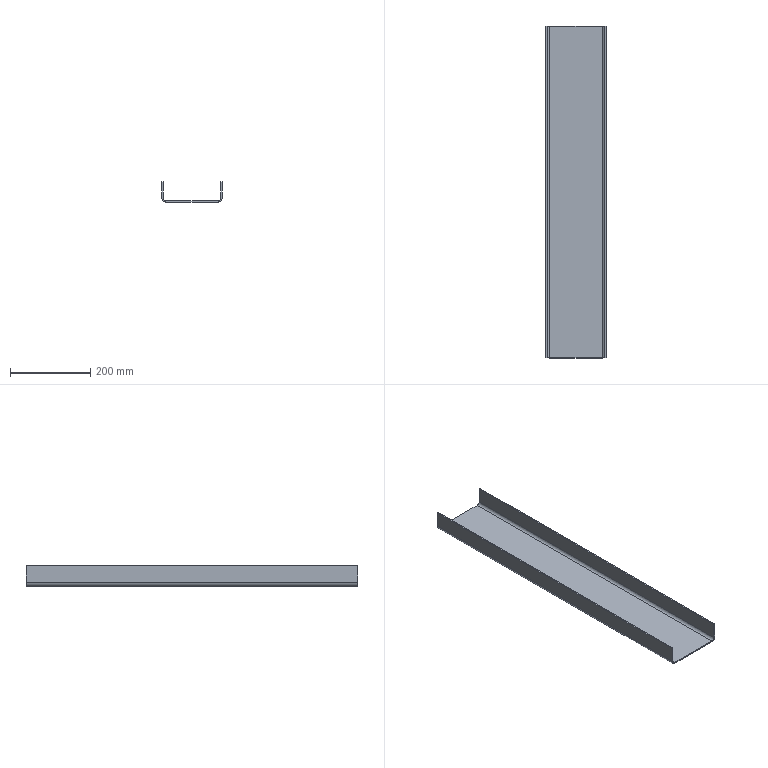Part | SolidWorks | features ExtruThin 1 | 1 solid | 14 faces | box 150 x 827 x 50 mm | volume 587261 mm3 | plane 10 | cylinder 4 | commonest cylinder face diameters 14 x2 20 x2
STEP:
#1=CARTESIAN_POINT('',(-75.,-413.5,-15.));
#2=VERTEX_POINT('',#1);
#3=CARTESIAN_POINT('',(-75.,-413.5,25.));
#4=VERTEX_POINT('',#3);
#5=CARTESIAN_POINT('',(-75.,-413.5,-15.));
#6=DIRECTION('',(0.,0.,1.));
#7=VECTOR('',#6,1000.);
#8=LINE('',#5,#7);
#9=EDGE_CURVE('',#2,#4,#8,.T.);
#10=ORIENTED_EDGE('',*,*,#9,.T.);
#11=CARTESIAN_POINT('',(-75.,413.5,25.));
#12=VERTEX_POINT('',#11);
#13=CARTESIAN_POINT('',(-75.,413.5,25.));
#14=DIRECTION('',(0.,-1.,0.));
#15=VECTOR('',#14,1000.);
#16=LINE('',#13,#15);
#17=EDGE_CURVE('',#12,#4,#16,.T.);
#18=ORIENTED_EDGE('',*,*,#17,.F.);
#19=CARTESIAN_POINT('',(-75.,413.5,-15.));
#20=VERTEX_POINT('',#19);
#21=CARTESIAN_POINT('',(-75.,413.5,-15.));
#22=DIRECTION('',(0.,0.,1.));
#23=VECTOR('',#22,1000.);
#24=LINE('',#21,#23);
#25=EDGE_CURVE('',#20,#12,#24,.T.);
#26=ORIENTED_EDGE('',*,*,#25,.F.);
#27=CARTESIAN_POINT('',(-75.,413.5,-15.));
#28=DIRECTION('',(0.,-1.,0.));
#29=VECTOR('',#28,1000.);
#30=LINE('',#27,#29);
#31=EDGE_CURVE('',#20,#2,#30,.T.);
#32=ORIENTED_EDGE('',*,*,#31,.T.);
#33=EDGE_LOOP('',(#10,#18,#26,#32));
#34=FACE_OUTER_BOUND('',#33,.T.);
#35=CARTESIAN_POINT('',(-75.,413.5,-15.));
#36=DIRECTION('',(1.,0.,0.));
#37=DIRECTION('',(0.,0.,-1.));
#38=AXIS2_PLACEMENT_3D('',#35,#36,#37);
#39=PLANE('',#38);
#40=ADVANCED_FACE('',(#34),#39,.F.);
#41=CARTESIAN_POINT('',(-72.,-413.5,25.));
#42=VERTEX_POINT('',#41);
#43=CARTESIAN_POINT('',(-72.,-413.5,25.));
#44=DIRECTION('',(-1.,0.,0.));
#45=VECTOR('',#44,1000.);
#46=LINE('',#43,#45);
#47=EDGE_CURVE('',#42,#4,#46,.T.);
#48=ORIENTED_EDGE('',*,*,#47,.F.);
#49=CARTESIAN_POINT('',(-72.,413.5,25.));
#50=VERTEX_POINT('',#49);
#51=CARTESIAN_POINT('',(-72.,413.5,25.));
#52=DIRECTION('',(0.,-1.,0.));
#53=VECTOR('',#52,1000.);
#54=LINE('',#51,#53);
#55=EDGE_CURVE('',#50,#42,#54,.T.);
#56=ORIENTED_EDGE('',*,*,#55,.F.);
#57=CARTESIAN_POINT('',(-72.,413.5,25.));
#58=DIRECTION('',(-1.,0.,0.));
#59=VECTOR('',#58,1000.);
#60=LINE('',#57,#59);
#61=EDGE_CURVE('',#50,#12,#60,.T.);
#62=ORIENTED_EDGE('',*,*,#61,.T.);
#63=ORIENTED_EDGE('',*,*,#17,.T.);
#64=EDGE_LOOP('',(#48,#56,#62,#63));
#65=FACE_OUTER_BOUND('',#64,.T.);
#66=CARTESIAN_POINT('',(-72.,413.5,25.));
#67=DIRECTION('',(0.,0.,1.));
#68=DIRECTION('',(1.,0.,0.));
#69=AXIS2_PLACEMENT_3D('',#66,#67,#68);
#70=PLANE('',#69);
#71=ADVANCED_FACE('',(#65),#70,.T.);
#72=CARTESIAN_POINT('',(-72.,-413.5,-15.));
#73=VERTEX_POINT('',#72);
#74=CARTESIAN_POINT('',(-72.,-413.5,-15.));
#75=DIRECTION('',(0.,0.,1.));
#76=VECTOR('',#75,1000.);
#77=LINE('',#74,#76);
#78=EDGE_CURVE('',#73,#42,#77,.T.);
#79=ORIENTED_EDGE('',*,*,#78,.F.);
#80=CARTESIAN_POINT('',(-72.,413.5,-15.));
#81=VERTEX_POINT('',#80);
#82=CARTESIAN_POINT('',(-72.,413.5,-15.));
#83=DIRECTION('',(0.,-1.,0.));
#84=VECTOR('',#83,1000.);
#85=LINE('',#82,#84);
#86=EDGE_CURVE('',#81,#73,#85,.T.);
#87=ORIENTED_EDGE('',*,*,#86,.F.);
#88=CARTESIAN_POINT('',(-72.,413.5,-15.));
#89=DIRECTION('',(0.,0.,1.));
#90=VECTOR('',#89,1000.);
#91=LINE('',#88,#90);
#92=EDGE_CURVE('',#81,#50,#91,.T.);
#93=ORIENTED_EDGE('',*,*,#92,.T.);
#94=ORIENTED_EDGE('',*,*,#55,.T.);
#95=EDGE_LOOP('',(#79,#87,#93,#94));
#96=FACE_OUTER_BOUND('',#95,.T.);
#97=CARTESIAN_POINT('',(-72.,413.5,-15.));
#98=DIRECTION('',(1.,0.,0.));
#99=DIRECTION('',(0.,0.,-1.));
#100=AXIS2_PLACEMENT_3D('',#97,#98,#99);
#101=PLANE('',#100);
#102=ADVANCED_FACE('',(#96),#101,.T.);
#103=CARTESIAN_POINT('',(-65.,-413.5,-22.));
#104=VERTEX_POINT('',#103);
#105=CARTESIAN_POINT('',(-65.,-413.5,-15.));
#106=DIRECTION('',(0.,1.,0.));
#107=DIRECTION('',(1.,0.,0.));
#108=AXIS2_PLACEMENT_3D('',#105,#106,#107);
#109=CIRCLE('',#108,7.);
#110=EDGE_CURVE('',#104,#73,#109,.T.);
#111=ORIENTED_EDGE('',*,*,#110,.F.);
#112=CARTESIAN_POINT('',(-65.,413.5,-22.));
#113=VERTEX_POINT('',#112);
#114=CARTESIAN_POINT('',(-65.,413.5,-22.));
#115=DIRECTION('',(0.,-1.,0.));
#116=VECTOR('',#115,1000.);
#117=LINE('',#114,#116);
#118=EDGE_CURVE('',#113,#104,#117,.T.);
#119=ORIENTED_EDGE('',*,*,#118,.F.);
#120=CARTESIAN_POINT('',(-65.,413.5,-15.));
#121=DIRECTION('',(0.,1.,0.));
#122=DIRECTION('',(1.,0.,0.));
#123=AXIS2_PLACEMENT_3D('',#120,#121,#122);
#124=CIRCLE('',#123,7.);
#125=EDGE_CURVE('',#113,#81,#124,.T.);
#126=ORIENTED_EDGE('',*,*,#125,.T.);
#127=ORIENTED_EDGE('',*,*,#86,.T.);
#128=EDGE_LOOP('',(#111,#119,#126,#127));
#129=FACE_OUTER_BOUND('',#128,.T.);
#130=CARTESIAN_POINT('',(-65.,413.5,-15.));
#131=DIRECTION('',(0.,-1.,0.));
#132=DIRECTION('',(0.,0.,-1.));
#133=AXIS2_PLACEMENT_3D('',#130,#131,#132);
#134=CYLINDRICAL_SURFACE('',#133,7.);
#135=ADVANCED_FACE('',(#129),#134,.F.);
#136=CARTESIAN_POINT('',(65.,-413.5,-22.));
#137=VERTEX_POINT('',#136);
#138=CARTESIAN_POINT('',(-65.,-413.5,-22.));
#139=DIRECTION('',(-1.,0.,0.));
#140=VECTOR('',#139,1000.);
#141=LINE('',#138,#140);
#142=EDGE_CURVE('',#137,#104,#141,.T.);
#143=ORIENTED_EDGE('',*,*,#142,.F.);
#144=CARTESIAN_POINT('',(65.,413.5,-22.));
#145=VERTEX_POINT('',#144);
#146=CARTESIAN_POINT('',(65.,413.5,-22.));
#147=DIRECTION('',(0.,-1.,0.));
#148=VECTOR('',#147,1000.);
#149=LINE('',#146,#148);
#150=EDGE_CURVE('',#145,#137,#149,.T.);
#151=ORIENTED_EDGE('',*,*,#150,.F.);
#152=CARTESIAN_POINT('',(-65.,413.5,-22.));
#153=DIRECTION('',(-1.,0.,0.));
#154=VECTOR('',#153,1000.);
#155=LINE('',#152,#154);
#156=EDGE_CURVE('',#145,#113,#155,.T.);
#157=ORIENTED_EDGE('',*,*,#156,.T.);
#158=ORIENTED_EDGE('',*,*,#118,.T.);
#159=EDGE_LOOP('',(#143,#151,#157,#158));
#160=FACE_OUTER_BOUND('',#159,.T.);
#161=CARTESIAN_POINT('',(-65.,413.5,-22.));
#162=DIRECTION('',(0.,0.,1.));
#163=DIRECTION('',(1.,0.,0.));
#164=AXIS2_PLACEMENT_3D('',#161,#162,#163);
#165=PLANE('',#164);
#166=ADVANCED_FACE('',(#160),#165,.T.);
#167=CARTESIAN_POINT('',(72.,-413.5,-15.));
#168=VERTEX_POINT('',#167);
#169=CARTESIAN_POINT('',(65.,-413.5,-15.));
#170=DIRECTION('',(0.,1.,0.));
#171=DIRECTION('',(1.,0.,0.));
#172=AXIS2_PLACEMENT_3D('',#169,#170,#171);
#173=CIRCLE('',#172,7.);
#174=EDGE_CURVE('',#168,#137,#173,.T.);
#175=ORIENTED_EDGE('',*,*,#174,.F.);
#176=CARTESIAN_POINT('',(72.,413.5,-15.));
#177=VERTEX_POINT('',#176);
#178=CARTESIAN_POINT('',(72.,413.5,-15.));
#179=DIRECTION('',(0.,-1.,0.));
#180=VECTOR('',#179,1000.);
#181=LINE('',#178,#180);
#182=EDGE_CURVE('',#177,#168,#181,.T.);
#183=ORIENTED_EDGE('',*,*,#182,.F.);
#184=CARTESIAN_POINT('',(65.,413.5,-15.));
#185=DIRECTION('',(0.,1.,0.));
#186=DIRECTION('',(1.,0.,0.));
#187=AXIS2_PLACEMENT_3D('',#184,#185,#186);
#188=CIRCLE('',#187,7.);
#189=EDGE_CURVE('',#177,#145,#188,.T.);
#190=ORIENTED_EDGE('',*,*,#189,.T.);
#191=ORIENTED_EDGE('',*,*,#150,.T.);
#192=EDGE_LOOP('',(#175,#183,#190,#191));
#193=FACE_OUTER_BOUND('',#192,.T.);
#194=CARTESIAN_POINT('',(65.,413.5,-15.));
#195=DIRECTION('',(0.,-1.,0.));
#196=DIRECTION('',(0.,0.,-1.));
#197=AXIS2_PLACEMENT_3D('',#194,#195,#196);
#198=CYLINDRICAL_SURFACE('',#197,7.);
#199=ADVANCED_FACE('',(#193),#198,.F.);
#200=CARTESIAN_POINT('',(72.,-413.5,25.));
#201=VERTEX_POINT('',#200);
#202=CARTESIAN_POINT('',(72.,-413.5,-15.));
#203=DIRECTION('',(0.,0.,-1.));
#204=VECTOR('',#203,1000.);
#205=LINE('',#202,#204);
#206=EDGE_CURVE('',#201,#168,#205,.T.);
#207=ORIENTED_EDGE('',*,*,#206,.F.);
#208=CARTESIAN_POINT('',(72.,413.5,25.));
#209=VERTEX_POINT('',#208);
#210=CARTESIAN_POINT('',(72.,413.5,25.));
#211=DIRECTION('',(0.,-1.,0.));
#212=VECTOR('',#211,1000.);
#213=LINE('',#210,#212);
#214=EDGE_CURVE('',#209,#201,#213,.T.);
#215=ORIENTED_EDGE('',*,*,#214,.F.);
#216=CARTESIAN_POINT('',(72.,413.5,-15.));
#217=DIRECTION('',(0.,0.,-1.));
#218=VECTOR('',#217,1000.);
#219=LINE('',#216,#218);
#220=EDGE_CURVE('',#209,#177,#219,.T.);
#221=ORIENTED_EDGE('',*,*,#220,.T.);
#222=ORIENTED_EDGE('',*,*,#182,.T.);
#223=EDGE_LOOP('',(#207,#215,#221,#222));
#224=FACE_OUTER_BOUND('',#223,.T.);
#225=CARTESIAN_POINT('',(72.,413.5,-15.));
#226=DIRECTION('',(-1.,0.,0.));
#227=DIRECTION('',(0.,0.,1.));
#228=AXIS2_PLACEMENT_3D('',#225,#226,#227);
#229=PLANE('',#228);
#230=ADVANCED_FACE('',(#224),#229,.T.);
#231=CARTESIAN_POINT('',(75.,-413.5,25.));
#232=VERTEX_POINT('',#231);
#233=CARTESIAN_POINT('',(75.,-413.5,25.));
#234=DIRECTION('',(-1.,0.,0.));
#235=VECTOR('',#234,1000.);
#236=LINE('',#233,#235);
#237=EDGE_CURVE('',#232,#201,#236,.T.);
#238=ORIENTED_EDGE('',*,*,#237,.F.);
#239=CARTESIAN_POINT('',(75.,413.5,25.));
#240=VERTEX_POINT('',#239);
#241=CARTESIAN_POINT('',(75.,413.5,25.));
#242=DIRECTION('',(0.,-1.,0.));
#243=VECTOR('',#242,1000.);
#244=LINE('',#241,#243);
#245=EDGE_CURVE('',#240,#232,#244,.T.);
#246=ORIENTED_EDGE('',*,*,#245,.F.);
#247=CARTESIAN_POINT('',(75.,413.5,25.));
#248=DIRECTION('',(-1.,0.,0.));
#249=VECTOR('',#248,1000.);
#250=LINE('',#247,#249);
#251=EDGE_CURVE('',#240,#209,#250,.T.);
#252=ORIENTED_EDGE('',*,*,#251,.T.);
#253=ORIENTED_EDGE('',*,*,#214,.T.);
#254=EDGE_LOOP('',(#238,#246,#252,#253));
#255=FACE_OUTER_BOUND('',#254,.T.);
#256=CARTESIAN_POINT('',(75.,413.5,25.));
#257=DIRECTION('',(0.,0.,1.));
#258=DIRECTION('',(1.,0.,0.));
#259=AXIS2_PLACEMENT_3D('',#256,#257,#258);
#260=PLANE('',#259);
#261=ADVANCED_FACE('',(#255),#260,.T.);
#262=CARTESIAN_POINT('',(75.,-413.5,-15.));
#263=VERTEX_POINT('',#262);
#264=CARTESIAN_POINT('',(75.,-413.5,-15.));
#265=DIRECTION('',(0.,0.,-1.));
#266=VECTOR('',#265,1000.);
#267=LINE('',#264,#266);
#268=EDGE_CURVE('',#232,#263,#267,.T.);
#269=ORIENTED_EDGE('',*,*,#268,.T.);
#270=CARTESIAN_POINT('',(75.,413.5,-15.));
#271=VERTEX_POINT('',#270);
#272=CARTESIAN_POINT('',(75.,413.5,-15.));
#273=DIRECTION('',(0.,-1.,0.));
#274=VECTOR('',#273,1000.);
#275=LINE('',#272,#274);
#276=EDGE_CURVE('',#271,#263,#275,.T.);
#277=ORIENTED_EDGE('',*,*,#276,.F.);
#278=CARTESIAN_POINT('',(75.,413.5,-15.));
#279=DIRECTION('',(0.,0.,-1.));
#280=VECTOR('',#279,1000.);
#281=LINE('',#278,#280);
#282=EDGE_CURVE('',#240,#271,#281,.T.);
#283=ORIENTED_EDGE('',*,*,#282,.F.);
#284=ORIENTED_EDGE('',*,*,#245,.T.);
#285=EDGE_LOOP('',(#269,#277,#283,#284));
#286=FACE_OUTER_BOUND('',#285,.T.);
#287=CARTESIAN_POINT('',(75.,413.5,-15.));
#288=DIRECTION('',(-1.,0.,0.));
#289=DIRECTION('',(0.,0.,1.));
#290=AXIS2_PLACEMENT_3D('',#287,#288,#289);
#291=PLANE('',#290);
#292=ADVANCED_FACE('',(#286),#291,.F.);
#293=CARTESIAN_POINT('',(65.,-413.5,-25.));
#294=VERTEX_POINT('',#293);
#295=CARTESIAN_POINT('',(65.,-413.5,-15.));
#296=DIRECTION('',(0.,1.,0.));
#297=DIRECTION('',(0.,0.,-1.));
#298=AXIS2_PLACEMENT_3D('',#295,#296,#297);
#299=CIRCLE('',#298,10.);
#300=EDGE_CURVE('',#263,#294,#299,.T.);
#301=ORIENTED_EDGE('',*,*,#300,.T.);
#302=CARTESIAN_POINT('',(65.,413.5,-25.));
#303=VERTEX_POINT('',#302);
#304=CARTESIAN_POINT('',(65.,413.5,-25.));
#305=DIRECTION('',(0.,-1.,0.));
#306=VECTOR('',#305,1000.);
#307=LINE('',#304,#306);
#308=EDGE_CURVE('',#303,#294,#307,.T.);
#309=ORIENTED_EDGE('',*,*,#308,.F.);
#310=CARTESIAN_POINT('',(65.,413.5,-15.));
#311=DIRECTION('',(0.,1.,0.));
#312=DIRECTION('',(0.,0.,-1.));
#313=AXIS2_PLACEMENT_3D('',#310,#311,#312);
#314=CIRCLE('',#313,10.);
#315=EDGE_CURVE('',#271,#303,#314,.T.);
#316=ORIENTED_EDGE('',*,*,#315,.F.);
#317=ORIENTED_EDGE('',*,*,#276,.T.);
#318=EDGE_LOOP('',(#301,#309,#316,#317));
#319=FACE_OUTER_BOUND('',#318,.T.);
#320=CARTESIAN_POINT('',(65.,413.5,-15.));
#321=DIRECTION('',(0.,-1.,0.));
#322=DIRECTION('',(0.,0.,-1.));
#323=AXIS2_PLACEMENT_3D('',#320,#321,#322);
#324=CYLINDRICAL_SURFACE('',#323,10.);
#325=ADVANCED_FACE('',(#319),#324,.T.);
#326=CARTESIAN_POINT('',(-65.,-413.5,-25.));
#327=VERTEX_POINT('',#326);
#328=CARTESIAN_POINT('',(-65.,-413.5,-25.));
#329=DIRECTION('',(-1.,0.,0.));
#330=VECTOR('',#329,1000.);
#331=LINE('',#328,#330);
#332=EDGE_CURVE('',#294,#327,#331,.T.);
#333=ORIENTED_EDGE('',*,*,#332,.T.);
#334=CARTESIAN_POINT('',(-65.,413.5,-25.));
#335=VERTEX_POINT('',#334);
#336=CARTESIAN_POINT('',(-65.,413.5,-25.));
#337=DIRECTION('',(0.,-1.,0.));
#338=VECTOR('',#337,1000.);
#339=LINE('',#336,#338);
#340=EDGE_CURVE('',#335,#327,#339,.T.);
#341=ORIENTED_EDGE('',*,*,#340,.F.);
#342=CARTESIAN_POINT('',(-65.,413.5,-25.));
#343=DIRECTION('',(-1.,0.,0.));
#344=VECTOR('',#343,1000.);
#345=LINE('',#342,#344);
#346=EDGE_CURVE('',#303,#335,#345,.T.);
#347=ORIENTED_EDGE('',*,*,#346,.F.);
#348=ORIENTED_EDGE('',*,*,#308,.T.);
#349=EDGE_LOOP('',(#333,#341,#347,#348));
#350=FACE_OUTER_BOUND('',#349,.T.);
#351=CARTESIAN_POINT('',(-65.,413.5,-25.));
#352=DIRECTION('',(0.,0.,1.));
#353=DIRECTION('',(1.,0.,0.));
#354=AXIS2_PLACEMENT_3D('',#351,#352,#353);
#355=PLANE('',#354);
#356=ADVANCED_FACE('',(#350),#355,.F.);
#357=CARTESIAN_POINT('',(-65.,-413.5,-15.));
#358=DIRECTION('',(0.,1.,0.));
#359=DIRECTION('',(0.,0.,1.));
#360=AXIS2_PLACEMENT_3D('',#357,#358,#359);
#361=CIRCLE('',#360,10.);
#362=EDGE_CURVE('',#327,#2,#361,.T.);
#363=ORIENTED_EDGE('',*,*,#362,.T.);
#364=ORIENTED_EDGE('',*,*,#31,.F.);
#365=CARTESIAN_POINT('',(-65.,413.5,-15.));
#366=DIRECTION('',(0.,1.,0.));
#367=DIRECTION('',(0.,0.,1.));
#368=AXIS2_PLACEMENT_3D('',#365,#366,#367);
#369=CIRCLE('',#368,10.);
#370=EDGE_CURVE('',#335,#20,#369,.T.);
#371=ORIENTED_EDGE('',*,*,#370,.F.);
#372=ORIENTED_EDGE('',*,*,#340,.T.);
#373=EDGE_LOOP('',(#363,#364,#371,#372));
#374=FACE_OUTER_BOUND('',#373,.T.);
#375=CARTESIAN_POINT('',(-65.,413.5,-15.));
#376=DIRECTION('',(0.,-1.,0.));
#377=DIRECTION('',(0.,0.,-1.));
#378=AXIS2_PLACEMENT_3D('',#375,#376,#377);
#379=CYLINDRICAL_SURFACE('',#378,10.);
#380=ADVANCED_FACE('',(#374),#379,.T.);
#381=ORIENTED_EDGE('',*,*,#25,.T.);
#382=ORIENTED_EDGE('',*,*,#61,.F.);
#383=ORIENTED_EDGE('',*,*,#92,.F.);
#384=ORIENTED_EDGE('',*,*,#125,.F.);
#385=ORIENTED_EDGE('',*,*,#156,.F.);
#386=ORIENTED_EDGE('',*,*,#189,.F.);
#387=ORIENTED_EDGE('',*,*,#220,.F.);
#388=ORIENTED_EDGE('',*,*,#251,.F.);
#389=ORIENTED_EDGE('',*,*,#282,.T.);
#390=ORIENTED_EDGE('',*,*,#315,.T.);
#391=ORIENTED_EDGE('',*,*,#346,.T.);
#392=ORIENTED_EDGE('',*,*,#370,.T.);
#393=EDGE_LOOP('',(#381,#382,#383,#384,#385,#386,#387,#388,#389,#390,#391,#392));
#394=FACE_OUTER_BOUND('',#393,.T.);
#395=CARTESIAN_POINT('',(-65.,413.5,-15.));
#396=DIRECTION('',(0.,1.,0.));
#397=DIRECTION('',(1.,0.,0.));
#398=AXIS2_PLACEMENT_3D('',#395,#396,#397);
#399=PLANE('',#398);
#400=ADVANCED_FACE('',(#394),#399,.T.);
#401=ORIENTED_EDGE('',*,*,#9,.F.);
#402=ORIENTED_EDGE('',*,*,#362,.F.);
#403=ORIENTED_EDGE('',*,*,#332,.F.);
#404=ORIENTED_EDGE('',*,*,#300,.F.);
#405=ORIENTED_EDGE('',*,*,#268,.F.);
#406=ORIENTED_EDGE('',*,*,#237,.T.);
#407=ORIENTED_EDGE('',*,*,#206,.T.);
#408=ORIENTED_EDGE('',*,*,#174,.T.);
#409=ORIENTED_EDGE('',*,*,#142,.T.);
#410=ORIENTED_EDGE('',*,*,#110,.T.);
#411=ORIENTED_EDGE('',*,*,#78,.T.);
#412=ORIENTED_EDGE('',*,*,#47,.T.);
#413=EDGE_LOOP('',(#401,#402,#403,#404,#405,#406,#407,#408,#409,#410,#411,#412));
#414=FACE_OUTER_BOUND('',#413,.T.);
#415=CARTESIAN_POINT('',(-65.,-413.5,-15.));
#416=DIRECTION('',(0.,1.,0.));
#417=DIRECTION('',(1.,0.,0.));
#418=AXIS2_PLACEMENT_3D('',#415,#416,#417);
#419=PLANE('',#418);
#420=ADVANCED_FACE('',(#414),#419,.F.);
#421=CLOSED_SHELL('',(#40,#71,#102,#135,#166,#199,#230,#261,#292,#325,#356,#380,#400,#420));
#422=MANIFOLD_SOLID_BREP('',#421);
#423=CARTESIAN_POINT('',(0.,0.,0.));
#424=DIRECTION('',(0.,0.,1.));
#425=DIRECTION('',(1.,0.,0.));
#426=AXIS2_PLACEMENT_3D('',#423,#424,#425);
#427=(LENGTH_UNIT()NAMED_UNIT(*)SI_UNIT(.MILLI.,.METRE.));
#428=UNCERTAINTY_MEASURE_WITH_UNIT(LENGTH_MEASURE(0.00001),#427,'','');
#429=(NAMED_UNIT(*)PLANE_ANGLE_UNIT()SI_UNIT($,.RADIAN.));
#430=(NAMED_UNIT(*)SI_UNIT($,.STERADIAN.)SOLID_ANGLE_UNIT());
#431=(GEOMETRIC_REPRESENTATION_CONTEXT(3)GLOBAL_UNCERTAINTY_ASSIGNED_CONTEXT((#428))GLOBAL_UNIT_ASSIGNED_CONTEXT((#427,#429,#430))REPRESENTATION_CONTEXT('',''));
#432=ADVANCED_BREP_SHAPE_REPRESENTATION('',(#422,#426),#431);